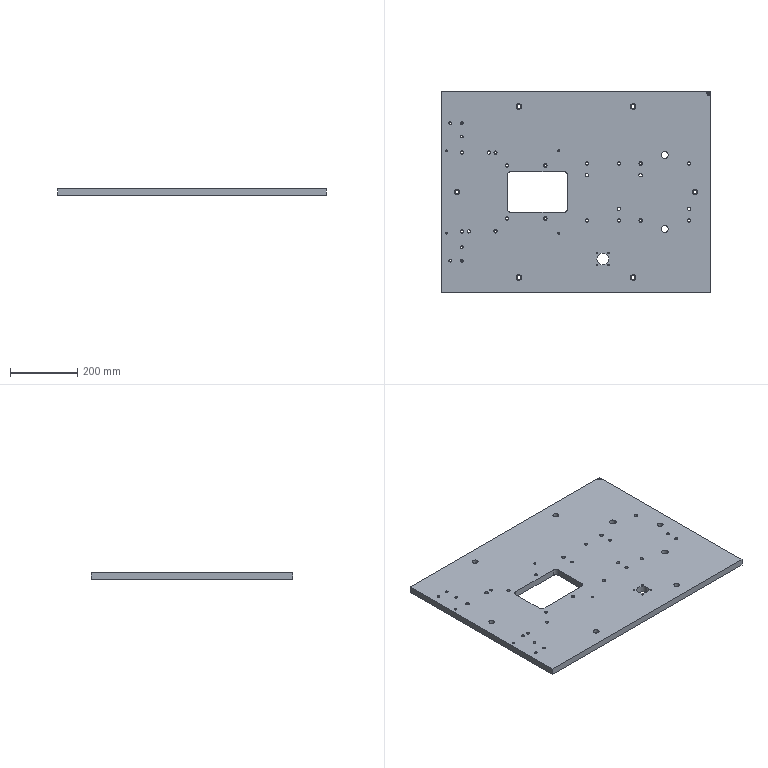Part | STEP file | 冲床-300配套压波_id1130_x_t | 1 solid | 134 faces | box 800 x 600 x 20 mm | volume 9083097 mm3 | cone 63 | cylinder 55 | plane 16 | commonest cylinder face diameters 8.5 x16 6.8 x6 10 x6 10.7 x6 17 x6 20 x6